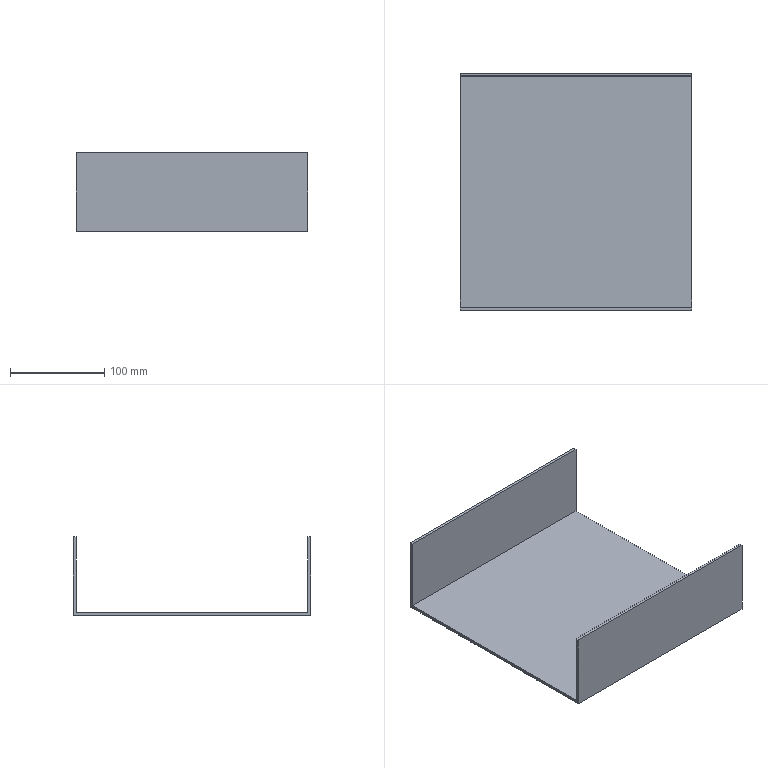Part | SolidWorks | features Extrusion 1, ICE 1 | 1 solid | 10 faces | box 246 x 252 x 83 mm | volume 304056 mm3 | plane 10
STEP:
#1=CARTESIAN_POINT('',(-123.,123.,3.));
#2=VERTEX_POINT('',#1);
#3=CARTESIAN_POINT('',(-123.,-123.,3.));
#4=VERTEX_POINT('',#3);
#5=CARTESIAN_POINT('',(-123.,126.,3.));
#6=DIRECTION('',(0.,-1.,0.));
#7=VECTOR('',#6,1000.);
#8=LINE('',#5,#7);
#9=EDGE_CURVE('',#2,#4,#8,.T.);
#10=ORIENTED_EDGE('',*,*,#9,.T.);
#11=CARTESIAN_POINT('',(123.,-123.,3.));
#12=VERTEX_POINT('',#11);
#13=CARTESIAN_POINT('',(123.,-123.,3.));
#14=DIRECTION('',(-1.,0.,0.));
#15=VECTOR('',#14,1000.);
#16=LINE('',#13,#15);
#17=EDGE_CURVE('',#12,#4,#16,.T.);
#18=ORIENTED_EDGE('',*,*,#17,.F.);
#19=CARTESIAN_POINT('',(123.,123.,3.));
#20=VERTEX_POINT('',#19);
#21=CARTESIAN_POINT('',(123.,126.,3.));
#22=DIRECTION('',(0.,1.,0.));
#23=VECTOR('',#22,1000.);
#24=LINE('',#21,#23);
#25=EDGE_CURVE('',#12,#20,#24,.T.);
#26=ORIENTED_EDGE('',*,*,#25,.T.);
#27=CARTESIAN_POINT('',(-123.,123.,3.));
#28=DIRECTION('',(1.,0.,0.));
#29=VECTOR('',#28,1000.);
#30=LINE('',#27,#29);
#31=EDGE_CURVE('',#2,#20,#30,.T.);
#32=ORIENTED_EDGE('',*,*,#31,.F.);
#33=EDGE_LOOP('',(#10,#18,#26,#32));
#34=FACE_OUTER_BOUND('',#33,.T.);
#35=CARTESIAN_POINT('',(0.,0.,3.));
#36=DIRECTION('',(0.,0.,1.));
#37=DIRECTION('',(1.,0.,0.));
#38=AXIS2_PLACEMENT_3D('',#35,#36,#37);
#39=PLANE('',#38);
#40=ADVANCED_FACE('',(#34),#39,.T.);
#41=CARTESIAN_POINT('',(123.,-126.,0.));
#42=VERTEX_POINT('',#41);
#43=CARTESIAN_POINT('',(123.,126.,0.));
#44=VERTEX_POINT('',#43);
#45=CARTESIAN_POINT('',(123.,126.,0.));
#46=DIRECTION('',(0.,1.,0.));
#47=VECTOR('',#46,1000.);
#48=LINE('',#45,#47);
#49=EDGE_CURVE('',#42,#44,#48,.T.);
#50=ORIENTED_EDGE('',*,*,#49,.T.);
#51=CARTESIAN_POINT('',(123.,126.,83.));
#52=VERTEX_POINT('',#51);
#53=CARTESIAN_POINT('',(123.,126.,3.));
#54=DIRECTION('',(0.,0.,-1.));
#55=VECTOR('',#54,1000.);
#56=LINE('',#53,#55);
#57=EDGE_CURVE('',#52,#44,#56,.T.);
#58=ORIENTED_EDGE('',*,*,#57,.F.);
#59=CARTESIAN_POINT('',(123.,123.,83.));
#60=VERTEX_POINT('',#59);
#61=CARTESIAN_POINT('',(123.,126.,83.));
#62=DIRECTION('',(0.,1.,0.));
#63=VECTOR('',#62,1000.);
#64=LINE('',#61,#63);
#65=EDGE_CURVE('',#60,#52,#64,.T.);
#66=ORIENTED_EDGE('',*,*,#65,.F.);
#67=CARTESIAN_POINT('',(123.,123.,83.));
#68=DIRECTION('',(0.,0.,-1.));
#69=VECTOR('',#68,1000.);
#70=LINE('',#67,#69);
#71=EDGE_CURVE('',#60,#20,#70,.T.);
#72=ORIENTED_EDGE('',*,*,#71,.T.);
#73=ORIENTED_EDGE('',*,*,#25,.F.);
#74=CARTESIAN_POINT('',(123.,-123.,83.));
#75=VERTEX_POINT('',#74);
#76=CARTESIAN_POINT('',(123.,-123.,83.));
#77=DIRECTION('',(0.,0.,-1.));
#78=VECTOR('',#77,1000.);
#79=LINE('',#76,#78);
#80=EDGE_CURVE('',#75,#12,#79,.T.);
#81=ORIENTED_EDGE('',*,*,#80,.F.);
#82=CARTESIAN_POINT('',(123.,-126.,83.));
#83=VERTEX_POINT('',#82);
#84=CARTESIAN_POINT('',(123.,-126.,83.));
#85=DIRECTION('',(0.,1.,0.));
#86=VECTOR('',#85,1000.);
#87=LINE('',#84,#86);
#88=EDGE_CURVE('',#83,#75,#87,.T.);
#89=ORIENTED_EDGE('',*,*,#88,.F.);
#90=CARTESIAN_POINT('',(123.,-126.,3.));
#91=DIRECTION('',(0.,0.,-1.));
#92=VECTOR('',#91,1000.);
#93=LINE('',#90,#92);
#94=EDGE_CURVE('',#83,#42,#93,.T.);
#95=ORIENTED_EDGE('',*,*,#94,.T.);
#96=EDGE_LOOP('',(#50,#58,#66,#72,#73,#81,#89,#95));
#97=FACE_OUTER_BOUND('',#96,.T.);
#98=CARTESIAN_POINT('',(123.,126.,3.));
#99=DIRECTION('',(-1.,0.,0.));
#100=DIRECTION('',(0.,-1.,0.));
#101=AXIS2_PLACEMENT_3D('',#98,#99,#100);
#102=PLANE('',#101);
#103=ADVANCED_FACE('',(#97),#102,.F.);
#104=CARTESIAN_POINT('',(-123.,126.,0.));
#105=VERTEX_POINT('',#104);
#106=CARTESIAN_POINT('',(-123.,126.,0.));
#107=DIRECTION('',(-1.,0.,0.));
#108=VECTOR('',#107,1000.);
#109=LINE('',#106,#108);
#110=EDGE_CURVE('',#44,#105,#109,.T.);
#111=ORIENTED_EDGE('',*,*,#110,.T.);
#112=CARTESIAN_POINT('',(-123.,126.,83.));
#113=VERTEX_POINT('',#112);
#114=CARTESIAN_POINT('',(-123.,126.,3.));
#115=DIRECTION('',(0.,0.,-1.));
#116=VECTOR('',#115,1000.);
#117=LINE('',#114,#116);
#118=EDGE_CURVE('',#113,#105,#117,.T.);
#119=ORIENTED_EDGE('',*,*,#118,.F.);
#120=CARTESIAN_POINT('',(-123.,126.,83.));
#121=DIRECTION('',(-1.,0.,0.));
#122=VECTOR('',#121,1000.);
#123=LINE('',#120,#122);
#124=EDGE_CURVE('',#52,#113,#123,.T.);
#125=ORIENTED_EDGE('',*,*,#124,.F.);
#126=ORIENTED_EDGE('',*,*,#57,.T.);
#127=EDGE_LOOP('',(#111,#119,#125,#126));
#128=FACE_OUTER_BOUND('',#127,.T.);
#129=CARTESIAN_POINT('',(-123.,126.,3.));
#130=DIRECTION('',(0.,-1.,0.));
#131=DIRECTION('',(0.,0.,-1.));
#132=AXIS2_PLACEMENT_3D('',#129,#130,#131);
#133=PLANE('',#132);
#134=ADVANCED_FACE('',(#128),#133,.F.);
#135=CARTESIAN_POINT('',(-123.,-126.,0.));
#136=VERTEX_POINT('',#135);
#137=CARTESIAN_POINT('',(-123.,126.,0.));
#138=DIRECTION('',(0.,-1.,0.));
#139=VECTOR('',#138,1000.);
#140=LINE('',#137,#139);
#141=EDGE_CURVE('',#105,#136,#140,.T.);
#142=ORIENTED_EDGE('',*,*,#141,.T.);
#143=CARTESIAN_POINT('',(-123.,-126.,83.));
#144=VERTEX_POINT('',#143);
#145=CARTESIAN_POINT('',(-123.,-126.,3.));
#146=DIRECTION('',(0.,0.,-1.));
#147=VECTOR('',#146,1000.);
#148=LINE('',#145,#147);
#149=EDGE_CURVE('',#144,#136,#148,.T.);
#150=ORIENTED_EDGE('',*,*,#149,.F.);
#151=CARTESIAN_POINT('',(-123.,-123.,83.));
#152=VERTEX_POINT('',#151);
#153=CARTESIAN_POINT('',(-123.,-126.,83.));
#154=DIRECTION('',(0.,-1.,0.));
#155=VECTOR('',#154,1000.);
#156=LINE('',#153,#155);
#157=EDGE_CURVE('',#152,#144,#156,.T.);
#158=ORIENTED_EDGE('',*,*,#157,.F.);
#159=CARTESIAN_POINT('',(-123.,-123.,83.));
#160=DIRECTION('',(0.,0.,-1.));
#161=VECTOR('',#160,1000.);
#162=LINE('',#159,#161);
#163=EDGE_CURVE('',#152,#4,#162,.T.);
#164=ORIENTED_EDGE('',*,*,#163,.T.);
#165=ORIENTED_EDGE('',*,*,#9,.F.);
#166=CARTESIAN_POINT('',(-123.,123.,83.));
#167=VERTEX_POINT('',#166);
#168=CARTESIAN_POINT('',(-123.,123.,83.));
#169=DIRECTION('',(0.,0.,-1.));
#170=VECTOR('',#169,1000.);
#171=LINE('',#168,#170);
#172=EDGE_CURVE('',#167,#2,#171,.T.);
#173=ORIENTED_EDGE('',*,*,#172,.F.);
#174=CARTESIAN_POINT('',(-123.,126.,83.));
#175=DIRECTION('',(0.,-1.,0.));
#176=VECTOR('',#175,1000.);
#177=LINE('',#174,#176);
#178=EDGE_CURVE('',#113,#167,#177,.T.);
#179=ORIENTED_EDGE('',*,*,#178,.F.);
#180=ORIENTED_EDGE('',*,*,#118,.T.);
#181=EDGE_LOOP('',(#142,#150,#158,#164,#165,#173,#179,#180));
#182=FACE_OUTER_BOUND('',#181,.T.);
#183=CARTESIAN_POINT('',(-123.,126.,3.));
#184=DIRECTION('',(1.,0.,0.));
#185=DIRECTION('',(0.,1.,0.));
#186=AXIS2_PLACEMENT_3D('',#183,#184,#185);
#187=PLANE('',#186);
#188=ADVANCED_FACE('',(#182),#187,.F.);
#189=CARTESIAN_POINT('',(-123.,-126.,0.));
#190=DIRECTION('',(1.,0.,0.));
#191=VECTOR('',#190,1000.);
#192=LINE('',#189,#191);
#193=EDGE_CURVE('',#136,#42,#192,.T.);
#194=ORIENTED_EDGE('',*,*,#193,.T.);
#195=ORIENTED_EDGE('',*,*,#94,.F.);
#196=CARTESIAN_POINT('',(123.,-126.,83.));
#197=DIRECTION('',(1.,0.,0.));
#198=VECTOR('',#197,1000.);
#199=LINE('',#196,#198);
#200=EDGE_CURVE('',#144,#83,#199,.T.);
#201=ORIENTED_EDGE('',*,*,#200,.F.);
#202=ORIENTED_EDGE('',*,*,#149,.T.);
#203=EDGE_LOOP('',(#194,#195,#201,#202));
#204=FACE_OUTER_BOUND('',#203,.T.);
#205=CARTESIAN_POINT('',(-123.,-126.,3.));
#206=DIRECTION('',(0.,1.,0.));
#207=DIRECTION('',(0.,0.,1.));
#208=AXIS2_PLACEMENT_3D('',#205,#206,#207);
#209=PLANE('',#208);
#210=ADVANCED_FACE('',(#204),#209,.F.);
#211=ORIENTED_EDGE('',*,*,#49,.F.);
#212=ORIENTED_EDGE('',*,*,#193,.F.);
#213=ORIENTED_EDGE('',*,*,#141,.F.);
#214=ORIENTED_EDGE('',*,*,#110,.F.);
#215=EDGE_LOOP('',(#211,#212,#213,#214));
#216=FACE_OUTER_BOUND('',#215,.T.);
#217=CARTESIAN_POINT('',(0.,0.,0.));
#218=DIRECTION('',(0.,0.,1.));
#219=DIRECTION('',(1.,0.,0.));
#220=AXIS2_PLACEMENT_3D('',#217,#218,#219);
#221=PLANE('',#220);
#222=ADVANCED_FACE('',(#216),#221,.F.);
#223=ORIENTED_EDGE('',*,*,#31,.T.);
#224=ORIENTED_EDGE('',*,*,#71,.F.);
#225=CARTESIAN_POINT('',(-123.,123.,83.));
#226=DIRECTION('',(1.,0.,0.));
#227=VECTOR('',#226,1000.);
#228=LINE('',#225,#227);
#229=EDGE_CURVE('',#167,#60,#228,.T.);
#230=ORIENTED_EDGE('',*,*,#229,.F.);
#231=ORIENTED_EDGE('',*,*,#172,.T.);
#232=EDGE_LOOP('',(#223,#224,#230,#231));
#233=FACE_OUTER_BOUND('',#232,.T.);
#234=CARTESIAN_POINT('',(-123.,123.,83.));
#235=DIRECTION('',(0.,1.,0.));
#236=DIRECTION('',(0.,0.,1.));
#237=AXIS2_PLACEMENT_3D('',#234,#235,#236);
#238=PLANE('',#237);
#239=ADVANCED_FACE('',(#233),#238,.F.);
#240=ORIENTED_EDGE('',*,*,#178,.T.);
#241=ORIENTED_EDGE('',*,*,#229,.T.);
#242=ORIENTED_EDGE('',*,*,#65,.T.);
#243=ORIENTED_EDGE('',*,*,#124,.T.);
#244=EDGE_LOOP('',(#240,#241,#242,#243));
#245=FACE_OUTER_BOUND('',#244,.T.);
#246=CARTESIAN_POINT('',(0.,0.,83.));
#247=DIRECTION('',(0.,0.,1.));
#248=DIRECTION('',(1.,0.,0.));
#249=AXIS2_PLACEMENT_3D('',#246,#247,#248);
#250=PLANE('',#249);
#251=ADVANCED_FACE('',(#245),#250,.T.);
#252=ORIENTED_EDGE('',*,*,#17,.T.);
#253=ORIENTED_EDGE('',*,*,#163,.F.);
#254=CARTESIAN_POINT('',(123.,-123.,83.));
#255=DIRECTION('',(-1.,0.,0.));
#256=VECTOR('',#255,1000.);
#257=LINE('',#254,#256);
#258=EDGE_CURVE('',#75,#152,#257,.T.);
#259=ORIENTED_EDGE('',*,*,#258,.F.);
#260=ORIENTED_EDGE('',*,*,#80,.T.);
#261=EDGE_LOOP('',(#252,#253,#259,#260));
#262=FACE_OUTER_BOUND('',#261,.T.);
#263=CARTESIAN_POINT('',(123.,-123.,83.));
#264=DIRECTION('',(0.,-1.,0.));
#265=DIRECTION('',(1.,0.,0.));
#266=AXIS2_PLACEMENT_3D('',#263,#264,#265);
#267=PLANE('',#266);
#268=ADVANCED_FACE('',(#262),#267,.F.);
#269=ORIENTED_EDGE('',*,*,#88,.T.);
#270=ORIENTED_EDGE('',*,*,#258,.T.);
#271=ORIENTED_EDGE('',*,*,#157,.T.);
#272=ORIENTED_EDGE('',*,*,#200,.T.);
#273=EDGE_LOOP('',(#269,#270,#271,#272));
#274=FACE_OUTER_BOUND('',#273,.T.);
#275=CARTESIAN_POINT('',(0.,0.,83.));
#276=DIRECTION('',(0.,0.,1.));
#277=DIRECTION('',(1.,0.,0.));
#278=AXIS2_PLACEMENT_3D('',#275,#276,#277);
#279=PLANE('',#278);
#280=ADVANCED_FACE('',(#274),#279,.T.);
#281=CLOSED_SHELL('',(#40,#103,#134,#188,#210,#222,#239,#251,#268,#280));
#282=MANIFOLD_SOLID_BREP('',#281);
#283=CARTESIAN_POINT('',(0.,0.,0.));
#284=DIRECTION('',(0.,0.,1.));
#285=DIRECTION('',(1.,0.,0.));
#286=AXIS2_PLACEMENT_3D('',#283,#284,#285);
#287=(LENGTH_UNIT()NAMED_UNIT(*)SI_UNIT(.MILLI.,.METRE.));
#288=UNCERTAINTY_MEASURE_WITH_UNIT(LENGTH_MEASURE(0.00001),#287,'','');
#289=(NAMED_UNIT(*)PLANE_ANGLE_UNIT()SI_UNIT($,.RADIAN.));
#290=(NAMED_UNIT(*)SI_UNIT($,.STERADIAN.)SOLID_ANGLE_UNIT());
#291=(GEOMETRIC_REPRESENTATION_CONTEXT(3)GLOBAL_UNCERTAINTY_ASSIGNED_CONTEXT((#288))GLOBAL_UNIT_ASSIGNED_CONTEXT((#287,#289,#290))REPRESENTATION_CONTEXT('',''));
#292=ADVANCED_BREP_SHAPE_REPRESENTATION('',(#282,#286),#291);